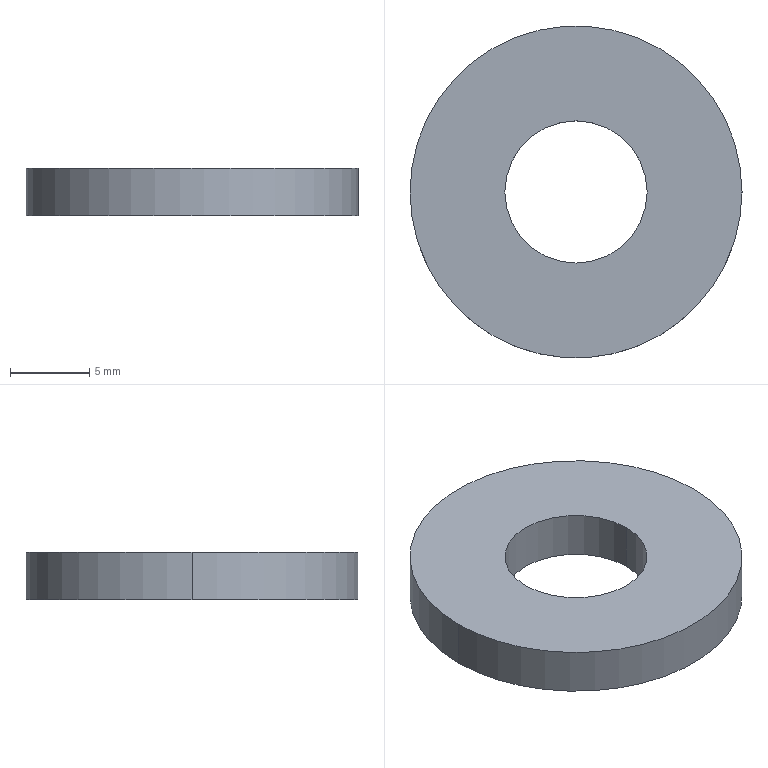Part | SolidWorks | features BaseBody 1 | 1 solid | 6 faces | box 21 x 21 x 3 mm | volume 848.23 mm3 | cylinder 4 | plane 2 | commonest cylinder face diameters 9 x2 21 x2
STEP:
#1=CARTESIAN_POINT('',(4.5,0.,3.));
#2=VERTEX_POINT('',#1);
#3=CARTESIAN_POINT('',(4.5,0.,0.));
#4=VERTEX_POINT('',#3);
#5=CARTESIAN_POINT('',(4.5,0.,3.));
#6=DIRECTION('',(0.,0.,-1.));
#7=VECTOR('',#6,1000.);
#8=LINE('',#5,#7);
#9=EDGE_CURVE('',#2,#4,#8,.T.);
#10=ORIENTED_EDGE('',*,*,#9,.F.);
#11=CARTESIAN_POINT('',(-4.5,0.,3.));
#12=VERTEX_POINT('',#11);
#13=CARTESIAN_POINT('',(0.,0.,3.));
#14=DIRECTION('',(0.,0.,1.));
#15=DIRECTION('',(1.,0.,0.));
#16=AXIS2_PLACEMENT_3D('',#13,#14,#15);
#17=CIRCLE('',#16,4.5);
#18=EDGE_CURVE('',#2,#12,#17,.T.);
#19=ORIENTED_EDGE('',*,*,#18,.T.);
#20=CARTESIAN_POINT('',(-4.5,0.,0.));
#21=VERTEX_POINT('',#20);
#22=CARTESIAN_POINT('',(-4.5,0.,3.));
#23=DIRECTION('',(0.,0.,-1.));
#24=VECTOR('',#23,1000.);
#25=LINE('',#22,#24);
#26=EDGE_CURVE('',#12,#21,#25,.T.);
#27=ORIENTED_EDGE('',*,*,#26,.T.);
#28=CARTESIAN_POINT('',(0.,0.,0.));
#29=DIRECTION('',(0.,0.,1.));
#30=DIRECTION('',(1.,0.,0.));
#31=AXIS2_PLACEMENT_3D('',#28,#29,#30);
#32=CIRCLE('',#31,4.5);
#33=EDGE_CURVE('',#4,#21,#32,.T.);
#34=ORIENTED_EDGE('',*,*,#33,.F.);
#35=EDGE_LOOP('',(#10,#19,#27,#34));
#36=FACE_OUTER_BOUND('',#35,.T.);
#37=CARTESIAN_POINT('',(0.,0.,3.));
#38=DIRECTION('',(0.,0.,-1.));
#39=DIRECTION('',(-1.,0.,0.));
#40=AXIS2_PLACEMENT_3D('',#37,#38,#39);
#41=CYLINDRICAL_SURFACE('',#40,4.5);
#42=ADVANCED_FACE('',(#36),#41,.F.);
#43=CARTESIAN_POINT('',(10.5,0.,3.));
#44=VERTEX_POINT('',#43);
#45=CARTESIAN_POINT('',(10.5,0.,0.));
#46=VERTEX_POINT('',#45);
#47=CARTESIAN_POINT('',(10.5,0.,3.));
#48=DIRECTION('',(0.,0.,-1.));
#49=VECTOR('',#48,1000.);
#50=LINE('',#47,#49);
#51=EDGE_CURVE('',#44,#46,#50,.T.);
#52=ORIENTED_EDGE('',*,*,#51,.F.);
#53=CARTESIAN_POINT('',(-10.5,0.,3.));
#54=VERTEX_POINT('',#53);
#55=CARTESIAN_POINT('',(0.,0.,3.));
#56=DIRECTION('',(0.,0.,1.));
#57=DIRECTION('',(1.,0.,0.));
#58=AXIS2_PLACEMENT_3D('',#55,#56,#57);
#59=CIRCLE('',#58,10.5);
#60=EDGE_CURVE('',#54,#44,#59,.T.);
#61=ORIENTED_EDGE('',*,*,#60,.F.);
#62=CARTESIAN_POINT('',(-10.5,0.,0.));
#63=VERTEX_POINT('',#62);
#64=CARTESIAN_POINT('',(-10.5,0.,3.));
#65=DIRECTION('',(0.,0.,-1.));
#66=VECTOR('',#65,1000.);
#67=LINE('',#64,#66);
#68=EDGE_CURVE('',#54,#63,#67,.T.);
#69=ORIENTED_EDGE('',*,*,#68,.T.);
#70=CARTESIAN_POINT('',(0.,0.,0.));
#71=DIRECTION('',(0.,0.,1.));
#72=DIRECTION('',(1.,0.,0.));
#73=AXIS2_PLACEMENT_3D('',#70,#71,#72);
#74=CIRCLE('',#73,10.5);
#75=EDGE_CURVE('',#63,#46,#74,.T.);
#76=ORIENTED_EDGE('',*,*,#75,.T.);
#77=EDGE_LOOP('',(#52,#61,#69,#76));
#78=FACE_OUTER_BOUND('',#77,.T.);
#79=CARTESIAN_POINT('',(0.,0.,3.));
#80=DIRECTION('',(0.,0.,-1.));
#81=DIRECTION('',(-1.,0.,0.));
#82=AXIS2_PLACEMENT_3D('',#79,#80,#81);
#83=CYLINDRICAL_SURFACE('',#82,10.5);
#84=ADVANCED_FACE('',(#78),#83,.T.);
#85=CARTESIAN_POINT('',(0.,0.,0.));
#86=DIRECTION('',(0.,0.,1.));
#87=DIRECTION('',(1.,0.,0.));
#88=AXIS2_PLACEMENT_3D('',#85,#86,#87);
#89=CIRCLE('',#88,4.5);
#90=EDGE_CURVE('',#21,#4,#89,.T.);
#91=ORIENTED_EDGE('',*,*,#90,.T.);
#92=ORIENTED_EDGE('',*,*,#33,.T.);
#93=EDGE_LOOP('',(#91,#92));
#94=FACE_BOUND('',#93,.T.);
#95=ORIENTED_EDGE('',*,*,#75,.F.);
#96=CARTESIAN_POINT('',(0.,0.,0.));
#97=DIRECTION('',(0.,0.,1.));
#98=DIRECTION('',(1.,0.,0.));
#99=AXIS2_PLACEMENT_3D('',#96,#97,#98);
#100=CIRCLE('',#99,10.5);
#101=EDGE_CURVE('',#46,#63,#100,.T.);
#102=ORIENTED_EDGE('',*,*,#101,.F.);
#103=EDGE_LOOP('',(#95,#102));
#104=FACE_OUTER_BOUND('',#103,.T.);
#105=CARTESIAN_POINT('',(0.,0.,0.));
#106=DIRECTION('',(0.,0.,1.));
#107=DIRECTION('',(1.,0.,0.));
#108=AXIS2_PLACEMENT_3D('',#105,#106,#107);
#109=PLANE('',#108);
#110=ADVANCED_FACE('',(#94,#104),#109,.F.);
#111=CARTESIAN_POINT('',(0.,0.,3.));
#112=DIRECTION('',(0.,0.,1.));
#113=DIRECTION('',(1.,0.,0.));
#114=AXIS2_PLACEMENT_3D('',#111,#112,#113);
#115=CIRCLE('',#114,4.5);
#116=EDGE_CURVE('',#12,#2,#115,.T.);
#117=ORIENTED_EDGE('',*,*,#116,.F.);
#118=ORIENTED_EDGE('',*,*,#18,.F.);
#119=EDGE_LOOP('',(#117,#118));
#120=FACE_BOUND('',#119,.T.);
#121=ORIENTED_EDGE('',*,*,#60,.T.);
#122=CARTESIAN_POINT('',(0.,0.,3.));
#123=DIRECTION('',(0.,0.,1.));
#124=DIRECTION('',(1.,0.,0.));
#125=AXIS2_PLACEMENT_3D('',#122,#123,#124);
#126=CIRCLE('',#125,10.5);
#127=EDGE_CURVE('',#44,#54,#126,.T.);
#128=ORIENTED_EDGE('',*,*,#127,.T.);
#129=EDGE_LOOP('',(#121,#128));
#130=FACE_OUTER_BOUND('',#129,.T.);
#131=CARTESIAN_POINT('',(0.,0.,3.));
#132=DIRECTION('',(0.,0.,1.));
#133=DIRECTION('',(1.,0.,0.));
#134=AXIS2_PLACEMENT_3D('',#131,#132,#133);
#135=PLANE('',#134);
#136=ADVANCED_FACE('',(#120,#130),#135,.T.);
#137=ORIENTED_EDGE('',*,*,#127,.F.);
#138=ORIENTED_EDGE('',*,*,#51,.T.);
#139=ORIENTED_EDGE('',*,*,#101,.T.);
#140=ORIENTED_EDGE('',*,*,#68,.F.);
#141=EDGE_LOOP('',(#137,#138,#139,#140));
#142=FACE_OUTER_BOUND('',#141,.T.);
#143=CARTESIAN_POINT('',(0.,0.,3.));
#144=DIRECTION('',(0.,0.,-1.));
#145=DIRECTION('',(-1.,0.,0.));
#146=AXIS2_PLACEMENT_3D('',#143,#144,#145);
#147=CYLINDRICAL_SURFACE('',#146,10.5);
#148=ADVANCED_FACE('',(#142),#147,.T.);
#149=ORIENTED_EDGE('',*,*,#116,.T.);
#150=ORIENTED_EDGE('',*,*,#9,.T.);
#151=ORIENTED_EDGE('',*,*,#90,.F.);
#152=ORIENTED_EDGE('',*,*,#26,.F.);
#153=EDGE_LOOP('',(#149,#150,#151,#152));
#154=FACE_OUTER_BOUND('',#153,.T.);
#155=CARTESIAN_POINT('',(0.,0.,3.));
#156=DIRECTION('',(0.,0.,-1.));
#157=DIRECTION('',(-1.,0.,0.));
#158=AXIS2_PLACEMENT_3D('',#155,#156,#157);
#159=CYLINDRICAL_SURFACE('',#158,4.5);
#160=ADVANCED_FACE('',(#154),#159,.F.);
#161=CLOSED_SHELL('',(#42,#84,#110,#136,#148,#160));
#162=MANIFOLD_SOLID_BREP('',#161);
#163=CARTESIAN_POINT('',(0.,0.,0.));
#164=DIRECTION('',(0.,0.,1.));
#165=DIRECTION('',(1.,0.,0.));
#166=AXIS2_PLACEMENT_3D('',#163,#164,#165);
#167=(LENGTH_UNIT()NAMED_UNIT(*)SI_UNIT(.MILLI.,.METRE.));
#168=UNCERTAINTY_MEASURE_WITH_UNIT(LENGTH_MEASURE(0.00001),#167,'','');
#169=(NAMED_UNIT(*)PLANE_ANGLE_UNIT()SI_UNIT($,.RADIAN.));
#170=(NAMED_UNIT(*)SI_UNIT($,.STERADIAN.)SOLID_ANGLE_UNIT());
#171=(GEOMETRIC_REPRESENTATION_CONTEXT(3)GLOBAL_UNCERTAINTY_ASSIGNED_CONTEXT((#168))GLOBAL_UNIT_ASSIGNED_CONTEXT((#167,#169,#170))REPRESENTATION_CONTEXT('',''));
#172=ADVANCED_BREP_SHAPE_REPRESENTATION('',(#162,#166),#171);